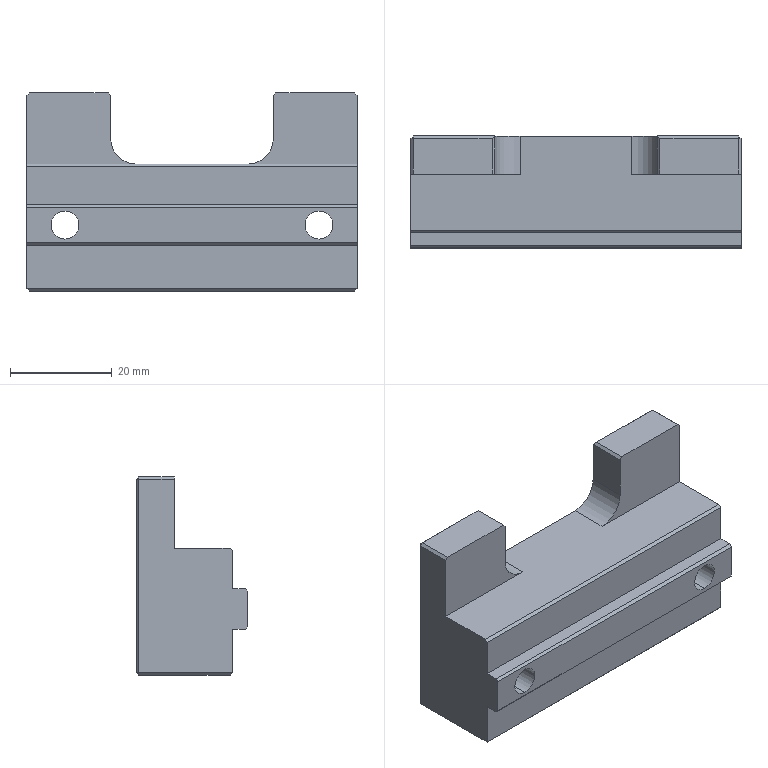Part | STEP file | PN_0008 fixture positioning plate 156 stations_Default | 1 solid | 54 faces | box 65 x 22 x 39 mm | volume 33983 mm3 | plane 37 | cylinder 14 | cone 3 | commonest cylinder face diameters 10 x6 4.2 x4 5.5 x4